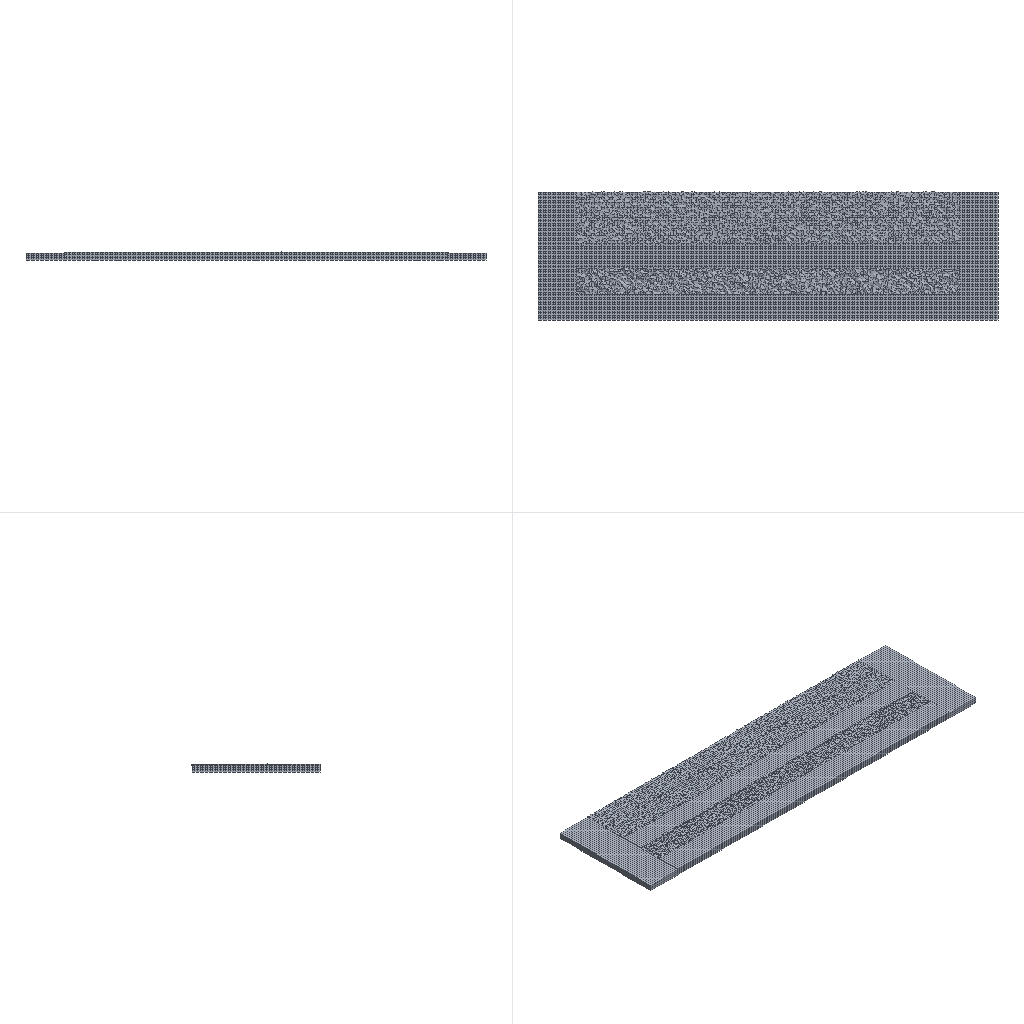Simulation study | abaqus
Set-up summary:
category,name,step,type,value,unit,region
solver,abaqus
solver,version,,,Abaqus/Standard 2020
units,not stated in the deck,,not stated
analysis,deck,,static,static
load_step,Step-1,Step-1,static,nlgeom=True
contact,interactions,,,general=0 pairs=0 ties=5
load_step,requested,,,1
mesh,nodes,,,39748
mesh,elements,,,27000
element_type,C3D8RH,,solid,27000
load,load commands in deck,,count,1
bc,support commands in deck,,count,7
material,MATERIAL-2,,in results
material,MATERIAL-2-COPY,,in results
check,setup vs results,,match,"per instance, exact: element labels, types and connectivity; labels of the nodes the elements use; coordinates of those nodes at SINGLE_PRECISION in 2 of 7 instance(s)"
Abaqus input file, long lists of numbers shortened:
*Heading
** Job name: 33212 Model name: 33212
** Generated by: Abaqus/CAE 2020
*Preprint, echo=NO, model=NO, history=NO, contact=NO
**
** PARTS
**
*Part, name=Part-510
*Node
      1,  0.04493,   -1.912,  0.6083
      2, 0.01957,  -1.782,  0.5905
** (6642 more lines like these left out)
*Element, type=C3D8RH
   1,   45,   46,   57,   56,    1,    2,   13,   12
   2,   46,   47,   58,   57,    2,    3,   14,   13
** (4498 more lines like these left out)
*Nset, nset=Set-2, generate
    1,  6644,     1
*Elset, elset=Set-2, generate
    1,  4500,     1
*Nset, nset=Set-3, generate
    1,  6644,     1
*Elset, elset=Set-3, generate
    1,  4500,     1
*Nset, nset=Set-1
    1,    2,    3,    4,    5,    6,    7,    8,    9,   10,   11,   45,   46,   47,   48,   49
   50,   51,   52,   53,   54,   55,   89,   90,   91,   92,   93,   94,   95,   96,   97,   98
** (102 more lines like these left out)
** Section: Section-2
*Solid Section, elset=Set-3, material=Material-2
,
*End Part
**
*Part, name=Part-550
*Node
      1, 0.03796,  -2.007,  0.5444
      2, -0.01504,  -1.801,  0.5905
** (6642 more lines like these left out)
*Element, type=C3D8RH
   1,   45,   46,   57,   56,    1,    2,   13,   12
   2,   46,   47,   58,   57,    2,    3,   14,   13
** (4498 more lines like these left out)
*Nset, nset=Set-2, generate
    1,  6644,     1
*Elset, elset=Set-2, generate
    1,  4500,     1
*Nset, nset=Set-3, generate
    1,  6644,     1
*Elset, elset=Set-3, generate
    1,  4500,     1
*Nset, nset=Set-1
    1,    2,    3,    4,    5,    6,    7,    8,    9,   10,   11,   45,   46,   47,   48,   49
   50,   51,   52,   53,   54,   55,   89,   90,   91,   92,   93,   94,   95,   96,   97,   98
** (102 more lines like these left out)
** Section: Section-2
*Solid Section, elset=Set-3, material=Material-2
,
*End Part
**
*Part, name=Part-600
*Node
      1,           0.,          -2.,  0.6
      2,           0.,  -1.8,  0.6
** (6642 more lines like these left out)
*Element, type=C3D8RH
   1,   45,   46,   57,   56,    1,    2,   13,   12
   2,   46,   47,   58,   57,    2,    3,   14,   13
** (4498 more lines like these left out)
*Nset, nset=Set-1, generate
    1,  6644,     1
*Elset, elset=Set-1, generate
    1,  4500,     1
*Nset, nset=Set-2, generate
    1,  6644,     1
*Elset, elset=Set-2, generate
    1,  4500,     1
** Section: Section-3
*Solid Section, elset=Set-2, material=Material-2-Copy
,
*End Part
**
*Part, name=Part-600-Copy
*Node
      1,          27.,         -10.,  0.52
      2,          27.,  -9.8,  0.52
** (3262 more lines like these left out)
*Element, type=C3D8RH
   1,  205,  206,  257,  256,    1,    2,   53,   52
   2,  206,  207,  258,  257,    2,    3,   54,   53
** (2248 more lines like these left out)
*Nset, nset=Set-1, generate
    1,  3264,     1
*Elset, elset=Set-1, generate
    1,  2250,     1
*Nset, nset=Set-2, generate
    1,  3264,     1
*Elset, elset=Set-2, generate
    1,  2250,     1
** Section: Section-3
*Solid Section, elset=Set-2, material=Material-2-Copy
,
*End Part
**
**
** ASSEMBLY
**
*Assembly, name=Assembly
**
*Instance, name=Part-550-1, part=Part-550
          0.,          -2.,           0.
*End Instance
**
*Instance, name=Part-600-2, part=Part-600
          0.,          -8.,           0.
*End Instance
**
*Instance, name=Part-510-2, part=Part-510
          0.,          -6.,           0.
*End Instance
**
*Instance, name=Part-600-Copy-1, part=Part-600-Copy
          3.,           0.,           0.
*End Instance
**
*Instance, name=Part-600-Copy-1-lin-2-1, part=Part-600-Copy
        -30.,           0.,           0.
*End Instance
**
*Instance, name=Part-600-2-lin-1-2, part=Part-600
          0.,          -4.,           0.
*End Instance
**
*Instance, name=Part-550-1-lin-1-2, part=Part-550
*End Instance
**
*Nset, nset=Set-6, instance=Part-600-Copy-1, generate
 3061,  3264,     1
*Elset, elset=Set-6, instance=Part-600-Copy-1, generate
 2101,  2250,     1
*Nset, nset=Set-7, instance=Part-600-Copy-1-lin-2-1, generate
   1,  204,    1
*Elset, elset=Set-7, instance=Part-600-Copy-1-lin-2-1, generate
   1,  150,    1
*Elset, elset=_m_Surf-17_S2, internal, instance=Part-600-Copy-1, generate
   1,  150,    1
*Elset, elset=_m_Surf-17_S1, internal, instance=Part-600-Copy-1-lin-2-1, generate
 2101,  2250,     1
*Surface, type=ELEMENT, name=m_Surf-17
_m_Surf-17_S2, S2
_m_Surf-17_S1, S1
*Elset, elset=_m_Surf-19_S4, internal, instance=Part-510-2, generate
   10,  4500,    10
*Surface, type=ELEMENT, name=m_Surf-19
_m_Surf-19_S4, S4
*Elset, elset=_m_Surf-21_S4, internal, instance=Part-600-2, generate
   10,  4500,    10
*Surface, type=ELEMENT, name=m_Surf-21
_m_Surf-21_S4, S4
*Elset, elset=_m_Surf-23_S4, internal, instance=Part-550-1, generate
   10,  4500,    10
*Surface, type=ELEMENT, name=m_Surf-23
_m_Surf-23_S4, S4
*Elset, elset=_m_Surf-30_S6, internal, instance=Part-550-1, generate
    1,  4491,    10
*Surface, type=ELEMENT, name=m_Surf-30
_m_Surf-30_S6, S6
*Elset, elset=_m_Surf-35_S4, internal, instance=Part-510-2, generate
   10,  4500,    10
*Surface, type=ELEMENT, name=m_Surf-35
_m_Surf-35_S4, S4
*Elset, elset=_s_Surf-17_S1, internal, instance=Part-550-1, generate
 4471,  4500,     1
*Elset, elset=_s_Surf-17_S1, internal, instance=Part-600-2, generate
 4471,  4500,     1
*Elset, elset=_s_Surf-17_S1, internal, instance=Part-510-2, generate
 4471,  4500,     1
*Elset, elset=_s_Surf-17_S2, internal, instance=Part-550-1, generate
  1,  30,   1
*Elset, elset=_s_Surf-17_S2, internal, instance=Part-600-2, generate
  1,  30,   1
*Elset, elset=_s_Surf-17_S2, internal, instance=Part-510-2, generate
  1,  30,   1
*Surface, type=ELEMENT, name=s_Surf-17
_s_Surf-17_S1, S1
_s_Surf-17_S2, S2
*Elset, elset=_s_Surf-19_S6, internal, instance=Part-600-2, generate
    1,  4491,    10
*Surface, type=ELEMENT, name=s_Surf-19
_s_Surf-19_S6, S6
*Elset, elset=_s_Surf-21_S6, internal, instance=Part-550-1, generate
    1,  4491,    10
*Surface, type=ELEMENT, name=s_Surf-21
_s_Surf-21_S6, S6
*Elset, elset=_s_Surf-27_S4, internal, instance=Part-510-2, generate
   10,  4500,    10
*Surface, type=ELEMENT, name=s_Surf-27
_s_Surf-27_S4, S4
*Elset, elset=_s_Surf-28_S6, internal, instance=Part-550-1, generate
    1,  4491,    10
*Surface, type=ELEMENT, name=s_Surf-28
_s_Surf-28_S6, S6
*Elset, elset=_s_Surf-29_S6, internal, instance=Part-510-2, generate
    1,  4491,    10
*Surface, type=ELEMENT, name=s_Surf-29
_s_Surf-29_S6, S6
*Elset, elset=_s_Surf-32_S1, internal, instance=Part-550-1, generate
 4471,  4500,     1
*Elset, elset=_s_Surf-32_S1, internal, instance=Part-600-2-lin-1-2, generate
 4471,  4500,     1
*Elset, elset=_s_Surf-32_S1, internal, instance=Part-550-1-lin-1-2, generate
 4471,  4500,     1
*Elset, elset=_s_Surf-32_S1, internal, instance=Part-600-2, generate
 4471,  4500,     1
*Elset, elset=_s_Surf-32_S1, internal, instance=Part-510-2, generate
 4471,  4500,     1
*Elset, elset=_s_Surf-32_S2, internal, instance=Part-550-1, generate
  1,  30,   1
*Elset, elset=_s_Surf-32_S2, internal, instance=Part-600-2-lin-1-2, generate
  1,  30,   1
*Elset, elset=_s_Surf-32_S2, internal, instance=Part-550-1-lin-1-2, generate
  1,  30,   1
*Elset, elset=_s_Surf-32_S2, internal, instance=Part-600-2, generate
  1,  30,   1
*Elset, elset=_s_Surf-32_S2, internal, instance=Part-510-2, generate
  1,  30,   1
*Surface, type=ELEMENT, name=s_Surf-32
_s_Surf-32_S1, S1
_s_Surf-32_S2, S2
*Elset, elset=_s_Surf-33_S6, internal, instance=Part-550-1-lin-1-2, generate
    1,  4491,    10
*Surface, type=ELEMENT, name=s_Surf-33
_s_Surf-33_S6, S6
*Elset, elset=_s_Surf-34_S4, internal, instance=Part-600-2-lin-1-2, generate
   10,  4500,    10
*Surface, type=ELEMENT, name=s_Surf-34
_s_Surf-34_S4, S4
*Elset, elset=_s_Surf-35_S6, internal, instance=Part-600-2-lin-1-2, generate
    1,  4491,    10
*Surface, type=ELEMENT, name=s_Surf-35
_s_Surf-35_S6, S6
** Constraint: Constraint-1
*Tie, name=Constraint-1, adjust=yes
s_Surf-32, m_Surf-17
** Constraint: Constraint-2
*Tie, name=Constraint-2, adjust=yes
s_Surf-35, m_Surf-35
** Constraint: Constraint-3
*Tie, name=Constraint-3, adjust=yes
s_Surf-29, m_Surf-21
** Constraint: Constraint-4
*Tie, name=Constraint-4, adjust=yes
s_Surf-33, m_Surf-23
** Constraint: Constraint-5
*Tie, name=Constraint-5, adjust=yes
s_Surf-34, m_Surf-30
*End Assembly
*Amplitude, name=Amp-1
             0.,              0.,              1.,              1.
**
** MATERIALS
**
*Material, name=Material-2
*Hyperelastic, mooney-rivlin
 0.144, 0.036,    0.
*Material, name=Material-2-Copy
*Hyperelastic, mooney-rivlin
 0.8, 0.19,   0.
** ----------------------------------------------------------------
**
** STEP: Step-1
**
*Step, name=Step-1, nlgeom=YES, inc=1000
*Static
0.01, 1., 1e-05, 0.1
**
** BOUNDARY CONDITIONS
**
** Name: BC-1 Type: 对称/反对称/完全固定
*Boundary
Set-6, ENCASTRE
** Name: BC-2 Type: 位移/转角
*Boundary, amplitude=Amp-1
Set-7, 1, 1, -15.
Set-7, 2, 2
Set-7, 3, 3
Set-7, 4, 4
Set-7, 5, 5
Set-7, 6, 6
**
** OUTPUT REQUESTS
**
*Restart, write, frequency=0
**
** FIELD OUTPUT: F-Output-1
**
*Output, field
*Node Output
CF, RF, RM, RT, U, V
*Element Output, directions=YES
E, LE, MISES, MISESMAX, NE, PE, PEEQ, PEEQMAX, PEEQT, PEMAG, PRESSONLY, S, SEQUT, YIELDPOT
*Contact Output
CDISP, CSTRESS
**
** HISTORY OUTPUT: H-Output-1
**
*Output, history, variable=PRESELECT
*End Step
Results summary:
result,step,,completed,increments=15 time=1.0/1.0
result,analysis,,,static
result,last_loadstep,,,1
result,analysis steps,,count,1
result,primary field,,,U
result,reaction total,,FX,0.0,model units
result,reaction total,,FY,-1e-06,model units
result,reaction total,,FZ,-0.0,model units